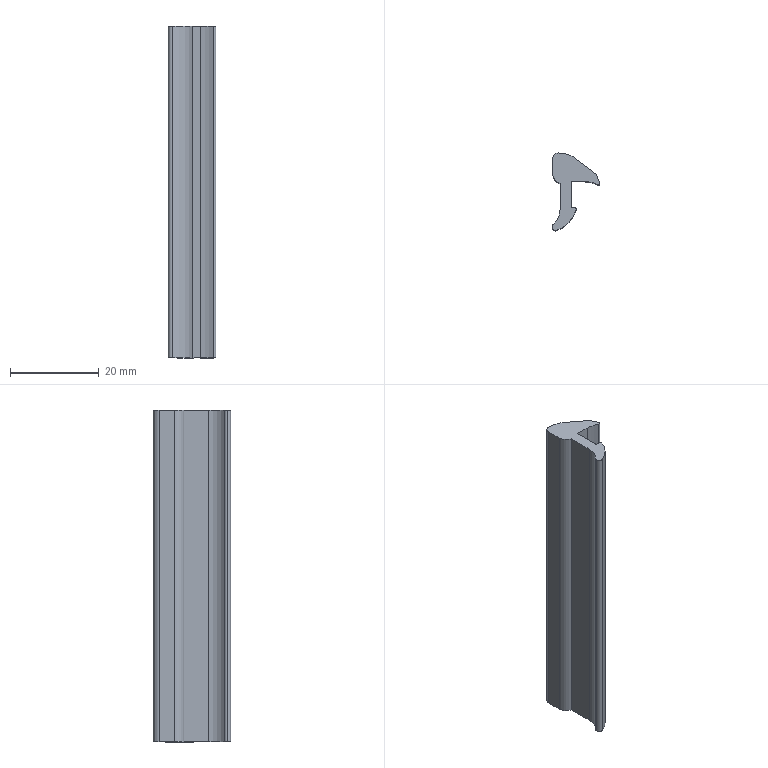Part | SolidWorks | features BaseBody 1, MoveFace 1 | 1 solid | 20 faces | box 10.8 x 17.5 x 75 mm | volume 5910 mm3 | cylinder 11 | plane 9 | commonest cylinder face diameters 1.6 x2 14 x2 0.4 x1 0.6 x1 0.8 x1 2.6 x1
STEP:
#1=CARTESIAN_POINT('',(-3.236,-11.055,-25.));
#2=VERTEX_POINT('',#1);
#3=CARTESIAN_POINT('',(-4.3,-10.3,-25.));
#4=VERTEX_POINT('',#3);
#5=CARTESIAN_POINT('',(-3.5,-10.3,-25.));
#6=DIRECTION('',(0.,0.,-1.));
#7=DIRECTION('',(1.,0.,0.));
#8=AXIS2_PLACEMENT_3D('',#5,#6,#7);
#9=CIRCLE('',#8,0.8);
#10=EDGE_CURVE('',#2,#4,#9,.T.);
#11=ORIENTED_EDGE('',*,*,#10,.T.);
#12=CARTESIAN_POINT('',(-4.3,-10.3,-100.));
#13=VERTEX_POINT('',#12);
#14=CARTESIAN_POINT('',(-4.3,-10.3,-100.));
#15=DIRECTION('',(0.,0.,-1.));
#16=VECTOR('',#15,1000.);
#17=LINE('',#14,#16);
#18=EDGE_CURVE('',#4,#13,#17,.T.);
#19=ORIENTED_EDGE('',*,*,#18,.T.);
#20=CARTESIAN_POINT('',(-3.236,-11.055,-100.));
#21=VERTEX_POINT('',#20);
#22=CARTESIAN_POINT('',(-3.5,-10.3,-100.));
#23=DIRECTION('',(0.,0.,1.));
#24=DIRECTION('',(-1.,0.,0.));
#25=AXIS2_PLACEMENT_3D('',#22,#23,#24);
#26=CIRCLE('',#25,0.8);
#27=EDGE_CURVE('',#13,#21,#26,.T.);
#28=ORIENTED_EDGE('',*,*,#27,.T.);
#29=CARTESIAN_POINT('',(-3.236,-11.055,-100.));
#30=DIRECTION('',(0.,0.,-1.));
#31=VECTOR('',#30,1000.);
#32=LINE('',#29,#31);
#33=EDGE_CURVE('',#2,#21,#32,.T.);
#34=ORIENTED_EDGE('',*,*,#33,.F.);
#35=EDGE_LOOP('',(#11,#19,#28,#34));
#36=FACE_OUTER_BOUND('',#35,.T.);
#37=CARTESIAN_POINT('',(-3.5,-10.3,-100.));
#38=DIRECTION('',(0.,0.,-1.));
#39=DIRECTION('',(-1.,0.,0.));
#40=AXIS2_PLACEMENT_3D('',#37,#38,#39);
#41=CYLINDRICAL_SURFACE('',#40,0.8);
#42=ADVANCED_FACE('',(#36),#41,.T.);
#43=CARTESIAN_POINT('',(1.184,-6.397,-100.));
#44=VERTEX_POINT('',#43);
#45=CARTESIAN_POINT('',(-5.702,-4.29,-100.));
#46=DIRECTION('',(0.,0.,1.));
#47=DIRECTION('',(-1.,0.,0.));
#48=AXIS2_PLACEMENT_3D('',#45,#46,#47);
#49=CIRCLE('',#48,7.201);
#50=EDGE_CURVE('',#21,#44,#49,.T.);
#51=ORIENTED_EDGE('',*,*,#50,.T.);
#52=CARTESIAN_POINT('',(1.184,-6.397,-25.));
#53=VERTEX_POINT('',#52);
#54=CARTESIAN_POINT('',(1.184,-6.397,-100.));
#55=DIRECTION('',(0.,0.,1.));
#56=VECTOR('',#55,1000.);
#57=LINE('',#54,#56);
#58=EDGE_CURVE('',#44,#53,#57,.T.);
#59=ORIENTED_EDGE('',*,*,#58,.T.);
#60=CARTESIAN_POINT('',(-5.702,-4.29,-25.));
#61=DIRECTION('',(0.,0.,-1.));
#62=DIRECTION('',(1.,0.,0.));
#63=AXIS2_PLACEMENT_3D('',#60,#61,#62);
#64=CIRCLE('',#63,7.201);
#65=EDGE_CURVE('',#53,#2,#64,.T.);
#66=ORIENTED_EDGE('',*,*,#65,.T.);
#67=ORIENTED_EDGE('',*,*,#33,.T.);
#68=EDGE_LOOP('',(#51,#59,#66,#67));
#69=FACE_OUTER_BOUND('',#68,.T.);
#70=CARTESIAN_POINT('',(-5.702,-4.29,-100.));
#71=DIRECTION('',(0.,0.,-1.));
#72=DIRECTION('',(-1.,0.,0.));
#73=AXIS2_PLACEMENT_3D('',#70,#71,#72);
#74=CYLINDRICAL_SURFACE('',#73,7.201);
#75=ADVANCED_FACE('',(#69),#74,.T.);
#76=CARTESIAN_POINT('',(0.9,-6.,-100.));
#77=VERTEX_POINT('',#76);
#78=CARTESIAN_POINT('',(0.9,-6.3,-100.));
#79=DIRECTION('',(0.,0.,1.));
#80=DIRECTION('',(-1.,0.,0.));
#81=AXIS2_PLACEMENT_3D('',#78,#79,#80);
#82=CIRCLE('',#81,0.3);
#83=EDGE_CURVE('',#44,#77,#82,.T.);
#84=ORIENTED_EDGE('',*,*,#83,.T.);
#85=CARTESIAN_POINT('',(0.9,-6.,-25.));
#86=VERTEX_POINT('',#85);
#87=CARTESIAN_POINT('',(0.9,-6.,-100.));
#88=DIRECTION('',(0.,0.,1.));
#89=VECTOR('',#88,1000.);
#90=LINE('',#87,#89);
#91=EDGE_CURVE('',#77,#86,#90,.T.);
#92=ORIENTED_EDGE('',*,*,#91,.T.);
#93=CARTESIAN_POINT('',(0.9,-6.3,-25.));
#94=DIRECTION('',(0.,0.,-1.));
#95=DIRECTION('',(1.,0.,0.));
#96=AXIS2_PLACEMENT_3D('',#93,#94,#95);
#97=CIRCLE('',#96,0.3);
#98=EDGE_CURVE('',#86,#53,#97,.T.);
#99=ORIENTED_EDGE('',*,*,#98,.T.);
#100=ORIENTED_EDGE('',*,*,#58,.F.);
#101=EDGE_LOOP('',(#84,#92,#99,#100));
#102=FACE_OUTER_BOUND('',#101,.T.);
#103=CARTESIAN_POINT('',(0.9,-6.3,-100.));
#104=DIRECTION('',(0.,0.,-1.));
#105=DIRECTION('',(-1.,0.,0.));
#106=AXIS2_PLACEMENT_3D('',#103,#104,#105);
#107=CYLINDRICAL_SURFACE('',#106,0.3);
#108=ADVANCED_FACE('',(#102),#107,.T.);
#109=CARTESIAN_POINT('',(-2.5,-0.5,-100.));
#110=VERTEX_POINT('',#109);
#111=CARTESIAN_POINT('',(-2.5,-6.153,-100.));
#112=VERTEX_POINT('',#111);
#113=CARTESIAN_POINT('',(-2.5,-6.397,-100.));
#114=DIRECTION('',(0.,-1.,0.));
#115=VECTOR('',#114,1000.);
#116=LINE('',#113,#115);
#117=EDGE_CURVE('',#110,#112,#116,.T.);
#118=ORIENTED_EDGE('',*,*,#117,.F.);
#119=CARTESIAN_POINT('',(-4.2,1.695,-100.));
#120=VERTEX_POINT('',#119);
#121=CARTESIAN_POINT('',(-1.701,1.875,-100.));
#122=DIRECTION('',(0.,0.,1.));
#123=DIRECTION('',(-1.,0.,0.));
#124=AXIS2_PLACEMENT_3D('',#121,#122,#123);
#125=CIRCLE('',#124,2.506);
#126=EDGE_CURVE('',#120,#110,#125,.T.);
#127=ORIENTED_EDGE('',*,*,#126,.F.);
#128=CARTESIAN_POINT('',(-4.2,5.1,-100.));
#129=VERTEX_POINT('',#128);
#130=CARTESIAN_POINT('',(-4.2,-6.397,-100.));
#131=DIRECTION('',(0.,-1.,0.));
#132=VECTOR('',#131,1000.);
#133=LINE('',#130,#132);
#134=EDGE_CURVE('',#129,#120,#133,.T.);
#135=ORIENTED_EDGE('',*,*,#134,.F.);
#136=CARTESIAN_POINT('',(-2.892,6.4,-100.));
#137=VERTEX_POINT('',#136);
#138=CARTESIAN_POINT('',(-2.9,5.1,-100.));
#139=DIRECTION('',(0.,0.,1.));
#140=DIRECTION('',(-1.,0.,0.));
#141=AXIS2_PLACEMENT_3D('',#138,#139,#140);
#142=CIRCLE('',#141,1.3);
#143=EDGE_CURVE('',#137,#129,#142,.T.);
#144=ORIENTED_EDGE('',*,*,#143,.F.);
#145=CARTESIAN_POINT('',(0.5,5.5,-100.));
#146=VERTEX_POINT('',#145);
#147=CARTESIAN_POINT('',(-2.934,-0.5999,-100.));
#148=DIRECTION('',(0.,0.,1.));
#149=DIRECTION('',(-1.,0.,0.));
#150=AXIS2_PLACEMENT_3D('',#147,#148,#149);
#151=CIRCLE('',#150,7.);
#152=EDGE_CURVE('',#146,#137,#151,.T.);
#153=ORIENTED_EDGE('',*,*,#152,.F.);
#154=CARTESIAN_POINT('',(5.5,1.7,-100.));
#155=VERTEX_POINT('',#154);
#156=CARTESIAN_POINT('',(5.5,1.7,-100.));
#157=DIRECTION('',(-0.7962,0.6051,0.));
#158=VECTOR('',#157,1000.);
#159=LINE('',#156,#158);
#160=EDGE_CURVE('',#155,#146,#159,.T.);
#161=ORIENTED_EDGE('',*,*,#160,.F.);
#162=CARTESIAN_POINT('',(6.458,-0.2215,-100.));
#163=VERTEX_POINT('',#162);
#164=CARTESIAN_POINT('',(6.458,-0.2215,-100.));
#165=DIRECTION('',(-0.4462,0.8949,0.));
#166=VECTOR('',#165,1000.);
#167=LINE('',#164,#166);
#168=EDGE_CURVE('',#163,#155,#167,.T.);
#169=ORIENTED_EDGE('',*,*,#168,.F.);
#170=CARTESIAN_POINT('',(5.895,-0.7433,-100.));
#171=VERTEX_POINT('',#170);
#172=CARTESIAN_POINT('',(6.1,-0.4,-100.));
#173=DIRECTION('',(0.,0.,1.));
#174=DIRECTION('',(-1.,0.,0.));
#175=AXIS2_PLACEMENT_3D('',#172,#173,#174);
#176=CIRCLE('',#175,0.4);
#177=EDGE_CURVE('',#171,#163,#176,.T.);
#178=ORIENTED_EDGE('',*,*,#177,.F.);
#179=CARTESIAN_POINT('',(3.,0.,-100.));
#180=VERTEX_POINT('',#179);
#181=CARTESIAN_POINT('',(2.746,-6.995,-100.));
#182=DIRECTION('',(0.,0.,-1.));
#183=DIRECTION('',(-1.,0.,0.));
#184=AXIS2_PLACEMENT_3D('',#181,#182,#183);
#185=CIRCLE('',#184,7.);
#186=EDGE_CURVE('',#180,#171,#185,.T.);
#187=ORIENTED_EDGE('',*,*,#186,.F.);
#188=CARTESIAN_POINT('',(0.,0.,-100.));
#189=VERTEX_POINT('',#188);
#190=CARTESIAN_POINT('',(-6.814,0.,-100.));
#191=DIRECTION('',(1.,0.,0.));
#192=VECTOR('',#191,1000.);
#193=LINE('',#190,#192);
#194=EDGE_CURVE('',#189,#180,#193,.T.);
#195=ORIENTED_EDGE('',*,*,#194,.F.);
#196=CARTESIAN_POINT('',(0.,-5.8,-100.));
#197=VERTEX_POINT('',#196);
#198=CARTESIAN_POINT('',(0.,-6.397,-100.));
#199=DIRECTION('',(0.,1.,0.));
#200=VECTOR('',#199,1000.);
#201=LINE('',#198,#200);
#202=EDGE_CURVE('',#197,#189,#201,.T.);
#203=ORIENTED_EDGE('',*,*,#202,.F.);
#204=CARTESIAN_POINT('',(0.2,-6.,-100.));
#205=VERTEX_POINT('',#204);
#206=CARTESIAN_POINT('',(0.2,-5.8,-100.));
#207=DIRECTION('',(0.,0.,1.));
#208=DIRECTION('',(-1.,0.,0.));
#209=AXIS2_PLACEMENT_3D('',#206,#207,#208);
#210=CIRCLE('',#209,0.2);
#211=EDGE_CURVE('',#197,#205,#210,.T.);
#212=ORIENTED_EDGE('',*,*,#211,.T.);
#213=CARTESIAN_POINT('',(-6.814,-6.,-100.));
#214=DIRECTION('',(-1.,0.,0.));
#215=VECTOR('',#214,1000.);
#216=LINE('',#213,#215);
#217=EDGE_CURVE('',#77,#205,#216,.T.);
#218=ORIENTED_EDGE('',*,*,#217,.F.);
#219=ORIENTED_EDGE('',*,*,#83,.F.);
#220=ORIENTED_EDGE('',*,*,#50,.F.);
#221=ORIENTED_EDGE('',*,*,#27,.F.);
#222=CARTESIAN_POINT('',(-3.998,-9.674,-100.));
#223=VERTEX_POINT('',#222);
#224=CARTESIAN_POINT('',(-3.5,-10.3,-100.));
#225=DIRECTION('',(0.,0.,1.));
#226=DIRECTION('',(-1.,0.,0.));
#227=AXIS2_PLACEMENT_3D('',#224,#225,#226);
#228=CIRCLE('',#227,0.8);
#229=EDGE_CURVE('',#223,#13,#228,.T.);
#230=ORIENTED_EDGE('',*,*,#229,.F.);
#231=CARTESIAN_POINT('',(-6.814,-6.397,-100.));
#232=DIRECTION('',(0.,0.,-1.));
#233=DIRECTION('',(-1.,0.,0.));
#234=AXIS2_PLACEMENT_3D('',#231,#232,#233);
#235=CIRCLE('',#234,4.321);
#236=EDGE_CURVE('',#112,#223,#235,.T.);
#237=ORIENTED_EDGE('',*,*,#236,.F.);
#238=EDGE_LOOP('',(#118,#127,#135,#144,#153,#161,#169,#178,#187,#195,#203,#212,#218,#219,#220,#221,#230,#237));
#239=FACE_OUTER_BOUND('',#238,.T.);
#240=CARTESIAN_POINT('',(-6.814,-6.397,-100.));
#241=DIRECTION('',(0.,0.,1.));
#242=DIRECTION('',(1.,0.,0.));
#243=AXIS2_PLACEMENT_3D('',#240,#241,#242);
#244=PLANE('',#243);
#245=ADVANCED_FACE('',(#239),#244,.F.);
#246=ORIENTED_EDGE('',*,*,#18,.F.);
#247=CARTESIAN_POINT('',(-3.998,-9.674,-25.));
#248=VERTEX_POINT('',#247);
#249=CARTESIAN_POINT('',(-3.5,-10.3,-25.));
#250=DIRECTION('',(0.,0.,-1.));
#251=DIRECTION('',(1.,0.,0.));
#252=AXIS2_PLACEMENT_3D('',#249,#250,#251);
#253=CIRCLE('',#252,0.8);
#254=EDGE_CURVE('',#4,#248,#253,.T.);
#255=ORIENTED_EDGE('',*,*,#254,.T.);
#256=CARTESIAN_POINT('',(-3.998,-9.674,-100.));
#257=DIRECTION('',(0.,0.,-1.));
#258=VECTOR('',#257,1000.);
#259=LINE('',#256,#258);
#260=EDGE_CURVE('',#248,#223,#259,.T.);
#261=ORIENTED_EDGE('',*,*,#260,.T.);
#262=ORIENTED_EDGE('',*,*,#229,.T.);
#263=EDGE_LOOP('',(#246,#255,#261,#262));
#264=FACE_OUTER_BOUND('',#263,.T.);
#265=CARTESIAN_POINT('',(-3.5,-10.3,-100.));
#266=DIRECTION('',(0.,0.,-1.));
#267=DIRECTION('',(-1.,0.,0.));
#268=AXIS2_PLACEMENT_3D('',#265,#266,#267);
#269=CYLINDRICAL_SURFACE('',#268,0.8);
#270=ADVANCED_FACE('',(#264),#269,.T.);
#271=CARTESIAN_POINT('',(-4.2,1.695,-25.));
#272=VERTEX_POINT('',#271);
#273=CARTESIAN_POINT('',(-2.5,-0.5,-25.));
#274=VERTEX_POINT('',#273);
#275=CARTESIAN_POINT('',(-1.701,1.875,-25.));
#276=DIRECTION('',(0.,0.,1.));
#277=DIRECTION('',(1.,0.,0.));
#278=AXIS2_PLACEMENT_3D('',#275,#276,#277);
#279=CIRCLE('',#278,2.506);
#280=EDGE_CURVE('',#272,#274,#279,.T.);
#281=ORIENTED_EDGE('',*,*,#280,.T.);
#282=CARTESIAN_POINT('',(-2.5,-6.153,-25.));
#283=VERTEX_POINT('',#282);
#284=CARTESIAN_POINT('',(-2.5,-6.397,-25.));
#285=DIRECTION('',(0.,-1.,0.));
#286=VECTOR('',#285,1000.);
#287=LINE('',#284,#286);
#288=EDGE_CURVE('',#274,#283,#287,.T.);
#289=ORIENTED_EDGE('',*,*,#288,.T.);
#290=CARTESIAN_POINT('',(-6.814,-6.397,-25.));
#291=DIRECTION('',(0.,0.,-1.));
#292=DIRECTION('',(1.,0.,0.));
#293=AXIS2_PLACEMENT_3D('',#290,#291,#292);
#294=CIRCLE('',#293,4.321);
#295=EDGE_CURVE('',#283,#248,#294,.T.);
#296=ORIENTED_EDGE('',*,*,#295,.T.);
#297=ORIENTED_EDGE('',*,*,#254,.F.);
#298=ORIENTED_EDGE('',*,*,#10,.F.);
#299=ORIENTED_EDGE('',*,*,#65,.F.);
#300=ORIENTED_EDGE('',*,*,#98,.F.);
#301=CARTESIAN_POINT('',(0.2,-6.,-25.));
#302=VERTEX_POINT('',#301);
#303=CARTESIAN_POINT('',(-6.814,-6.,-25.));
#304=DIRECTION('',(-1.,0.,0.));
#305=VECTOR('',#304,1000.);
#306=LINE('',#303,#305);
#307=EDGE_CURVE('',#86,#302,#306,.T.);
#308=ORIENTED_EDGE('',*,*,#307,.T.);
#309=CARTESIAN_POINT('',(0.,-5.8,-25.));
#310=VERTEX_POINT('',#309);
#311=CARTESIAN_POINT('',(0.2,-5.8,-25.));
#312=DIRECTION('',(0.,0.,-1.));
#313=DIRECTION('',(1.,0.,0.));
#314=AXIS2_PLACEMENT_3D('',#311,#312,#313);
#315=CIRCLE('',#314,0.2);
#316=EDGE_CURVE('',#302,#310,#315,.T.);
#317=ORIENTED_EDGE('',*,*,#316,.T.);
#318=CARTESIAN_POINT('',(0.,0.,-25.));
#319=VERTEX_POINT('',#318);
#320=CARTESIAN_POINT('',(0.,-6.397,-25.));
#321=DIRECTION('',(0.,1.,0.));
#322=VECTOR('',#321,1000.);
#323=LINE('',#320,#322);
#324=EDGE_CURVE('',#310,#319,#323,.T.);
#325=ORIENTED_EDGE('',*,*,#324,.T.);
#326=CARTESIAN_POINT('',(3.,0.,-25.));
#327=VERTEX_POINT('',#326);
#328=CARTESIAN_POINT('',(-6.814,0.,-25.));
#329=DIRECTION('',(1.,0.,0.));
#330=VECTOR('',#329,1000.);
#331=LINE('',#328,#330);
#332=EDGE_CURVE('',#319,#327,#331,.T.);
#333=ORIENTED_EDGE('',*,*,#332,.T.);
#334=CARTESIAN_POINT('',(5.895,-0.7433,-25.));
#335=VERTEX_POINT('',#334);
#336=CARTESIAN_POINT('',(2.746,-6.995,-25.));
#337=DIRECTION('',(0.,0.,-1.));
#338=DIRECTION('',(1.,0.,0.));
#339=AXIS2_PLACEMENT_3D('',#336,#337,#338);
#340=CIRCLE('',#339,7.);
#341=EDGE_CURVE('',#327,#335,#340,.T.);
#342=ORIENTED_EDGE('',*,*,#341,.T.);
#343=CARTESIAN_POINT('',(6.458,-0.2215,-25.));
#344=VERTEX_POINT('',#343);
#345=CARTESIAN_POINT('',(6.1,-0.4,-25.));
#346=DIRECTION('',(0.,0.,-1.));
#347=DIRECTION('',(1.,0.,0.));
#348=AXIS2_PLACEMENT_3D('',#345,#346,#347);
#349=CIRCLE('',#348,0.4);
#350=EDGE_CURVE('',#344,#335,#349,.T.);
#351=ORIENTED_EDGE('',*,*,#350,.F.);
#352=CARTESIAN_POINT('',(5.5,1.7,-25.));
#353=VERTEX_POINT('',#352);
#354=CARTESIAN_POINT('',(6.282,0.1323,-25.));
#355=DIRECTION('',(-0.4462,0.8949,0.));
#356=VECTOR('',#355,1000.);
#357=LINE('',#354,#356);
#358=EDGE_CURVE('',#344,#353,#357,.T.);
#359=ORIENTED_EDGE('',*,*,#358,.T.);
#360=CARTESIAN_POINT('',(0.5,5.5,-25.));
#361=VERTEX_POINT('',#360);
#362=CARTESIAN_POINT('',(1.595,4.668,-25.));
#363=DIRECTION('',(-0.7962,0.6051,0.));
#364=VECTOR('',#363,1000.);
#365=LINE('',#362,#364);
#366=EDGE_CURVE('',#353,#361,#365,.T.);
#367=ORIENTED_EDGE('',*,*,#366,.T.);
#368=CARTESIAN_POINT('',(-2.892,6.4,-25.));
#369=VERTEX_POINT('',#368);
#370=CARTESIAN_POINT('',(-2.934,-0.5999,-25.));
#371=DIRECTION('',(0.,0.,1.));
#372=DIRECTION('',(1.,0.,0.));
#373=AXIS2_PLACEMENT_3D('',#370,#371,#372);
#374=CIRCLE('',#373,7.);
#375=EDGE_CURVE('',#361,#369,#374,.T.);
#376=ORIENTED_EDGE('',*,*,#375,.T.);
#377=CARTESIAN_POINT('',(-4.2,5.1,-25.));
#378=VERTEX_POINT('',#377);
#379=CARTESIAN_POINT('',(-2.9,5.1,-25.));
#380=DIRECTION('',(0.,0.,1.));
#381=DIRECTION('',(1.,0.,0.));
#382=AXIS2_PLACEMENT_3D('',#379,#380,#381);
#383=CIRCLE('',#382,1.3);
#384=EDGE_CURVE('',#369,#378,#383,.T.);
#385=ORIENTED_EDGE('',*,*,#384,.T.);
#386=CARTESIAN_POINT('',(-4.2,-6.397,-25.));
#387=DIRECTION('',(0.,-1.,0.));
#388=VECTOR('',#387,1000.);
#389=LINE('',#386,#388);
#390=EDGE_CURVE('',#378,#272,#389,.T.);
#391=ORIENTED_EDGE('',*,*,#390,.T.);
#392=EDGE_LOOP('',(#281,#289,#296,#297,#298,#299,#300,#308,#317,#325,#333,#342,#351,#359,#367,#376,#385,#391));
#393=FACE_OUTER_BOUND('',#392,.T.);
#394=CARTESIAN_POINT('',(-6.814,-6.397,-25.));
#395=DIRECTION('',(0.,0.,1.));
#396=DIRECTION('',(1.,0.,0.));
#397=AXIS2_PLACEMENT_3D('',#394,#395,#396);
#398=PLANE('',#397);
#399=ADVANCED_FACE('',(#393),#398,.T.);
#400=ORIENTED_EDGE('',*,*,#217,.T.);
#401=CARTESIAN_POINT('',(0.2,-6.,-100.));
#402=DIRECTION('',(0.,0.,1.));
#403=VECTOR('',#402,1000.);
#404=LINE('',#401,#403);
#405=EDGE_CURVE('',#205,#302,#404,.T.);
#406=ORIENTED_EDGE('',*,*,#405,.T.);
#407=ORIENTED_EDGE('',*,*,#307,.F.);
#408=ORIENTED_EDGE('',*,*,#91,.F.);
#409=EDGE_LOOP('',(#400,#406,#407,#408));
#410=FACE_OUTER_BOUND('',#409,.T.);
#411=CARTESIAN_POINT('',(0.9,-6.,-100.));
#412=DIRECTION('',(0.,1.,0.));
#413=DIRECTION('',(0.,0.,1.));
#414=AXIS2_PLACEMENT_3D('',#411,#412,#413);
#415=PLANE('',#414);
#416=ADVANCED_FACE('',(#410),#415,.T.);
#417=CARTESIAN_POINT('',(-2.5,-6.153,-100.));
#418=DIRECTION('',(0.,0.,1.));
#419=VECTOR('',#418,1000.);
#420=LINE('',#417,#419);
#421=EDGE_CURVE('',#112,#283,#420,.T.);
#422=ORIENTED_EDGE('',*,*,#421,.F.);
#423=ORIENTED_EDGE('',*,*,#236,.T.);
#424=ORIENTED_EDGE('',*,*,#260,.F.);
#425=ORIENTED_EDGE('',*,*,#295,.F.);
#426=EDGE_LOOP('',(#422,#423,#424,#425));
#427=FACE_OUTER_BOUND('',#426,.T.);
#428=CARTESIAN_POINT('',(-6.814,-6.397,-100.));
#429=DIRECTION('',(0.,0.,-1.));
#430=DIRECTION('',(-1.,0.,0.));
#431=AXIS2_PLACEMENT_3D('',#428,#429,#430);
#432=CYLINDRICAL_SURFACE('',#431,4.321);
#433=ADVANCED_FACE('',(#427),#432,.F.);
#434=ORIENTED_EDGE('',*,*,#117,.T.);
#435=ORIENTED_EDGE('',*,*,#421,.T.);
#436=ORIENTED_EDGE('',*,*,#288,.F.);
#437=CARTESIAN_POINT('',(-2.5,-0.5,-100.));
#438=DIRECTION('',(0.,0.,-1.));
#439=VECTOR('',#438,1000.);
#440=LINE('',#437,#439);
#441=EDGE_CURVE('',#274,#110,#440,.T.);
#442=ORIENTED_EDGE('',*,*,#441,.T.);
#443=EDGE_LOOP('',(#434,#435,#436,#442));
#444=FACE_OUTER_BOUND('',#443,.T.);
#445=CARTESIAN_POINT('',(-2.5,-0.5,-100.));
#446=DIRECTION('',(-1.,0.,0.));
#447=DIRECTION('',(0.,0.,1.));
#448=AXIS2_PLACEMENT_3D('',#445,#446,#447);
#449=PLANE('',#448);
#450=ADVANCED_FACE('',(#444),#449,.T.);
#451=ORIENTED_EDGE('',*,*,#126,.T.);
#452=ORIENTED_EDGE('',*,*,#441,.F.);
#453=ORIENTED_EDGE('',*,*,#280,.F.);
#454=CARTESIAN_POINT('',(-4.2,1.695,-100.));
#455=DIRECTION('',(0.,0.,-1.));
#456=VECTOR('',#455,1000.);
#457=LINE('',#454,#456);
#458=EDGE_CURVE('',#272,#120,#457,.T.);
#459=ORIENTED_EDGE('',*,*,#458,.T.);
#460=EDGE_LOOP('',(#451,#452,#453,#459));
#461=FACE_OUTER_BOUND('',#460,.T.);
#462=CARTESIAN_POINT('',(-1.701,1.875,-100.));
#463=DIRECTION('',(0.,0.,-1.));
#464=DIRECTION('',(-1.,0.,0.));
#465=AXIS2_PLACEMENT_3D('',#462,#463,#464);
#466=CYLINDRICAL_SURFACE('',#465,2.506);
#467=ADVANCED_FACE('',(#461),#466,.T.);
#468=ORIENTED_EDGE('',*,*,#134,.T.);
#469=ORIENTED_EDGE('',*,*,#458,.F.);
#470=ORIENTED_EDGE('',*,*,#390,.F.);
#471=CARTESIAN_POINT('',(-4.2,5.1,-100.));
#472=DIRECTION('',(0.,0.,-1.));
#473=VECTOR('',#472,1000.);
#474=LINE('',#471,#473);
#475=EDGE_CURVE('',#378,#129,#474,.T.);
#476=ORIENTED_EDGE('',*,*,#475,.T.);
#477=EDGE_LOOP('',(#468,#469,#470,#476));
#478=FACE_OUTER_BOUND('',#477,.T.);
#479=CARTESIAN_POINT('',(-4.2,5.1,-100.));
#480=DIRECTION('',(-1.,0.,0.));
#481=DIRECTION('',(0.,0.,1.));
#482=AXIS2_PLACEMENT_3D('',#479,#480,#481);
#483=PLANE('',#482);
#484=ADVANCED_FACE('',(#478),#483,.T.);
#485=ORIENTED_EDGE('',*,*,#143,.T.);
#486=ORIENTED_EDGE('',*,*,#475,.F.);
#487=ORIENTED_EDGE('',*,*,#384,.F.);
#488=CARTESIAN_POINT('',(-2.892,6.4,-100.));
#489=DIRECTION('',(0.,0.,-1.));
#490=VECTOR('',#489,1000.);
#491=LINE('',#488,#490);
#492=EDGE_CURVE('',#369,#137,#491,.T.);
#493=ORIENTED_EDGE('',*,*,#492,.T.);
#494=EDGE_LOOP('',(#485,#486,#487,#493));
#495=FACE_OUTER_BOUND('',#494,.T.);
#496=CARTESIAN_POINT('',(-2.9,5.1,-100.));
#497=DIRECTION('',(0.,0.,-1.));
#498=DIRECTION('',(-1.,0.,0.));
#499=AXIS2_PLACEMENT_3D('',#496,#497,#498);
#500=CYLINDRICAL_SURFACE('',#499,1.3);
#501=ADVANCED_FACE('',(#495),#500,.T.);
#502=ORIENTED_EDGE('',*,*,#152,.T.);
#503=ORIENTED_EDGE('',*,*,#492,.F.);
#504=ORIENTED_EDGE('',*,*,#375,.F.);
#505=CARTESIAN_POINT('',(0.5,5.5,-100.));
#506=DIRECTION('',(0.,0.,-1.));
#507=VECTOR('',#506,1000.);
#508=LINE('',#505,#507);
#509=EDGE_CURVE('',#361,#146,#508,.T.);
#510=ORIENTED_EDGE('',*,*,#509,.T.);
#511=EDGE_LOOP('',(#502,#503,#504,#510));
#512=FACE_OUTER_BOUND('',#511,.T.);
#513=CARTESIAN_POINT('',(-2.934,-0.5999,-100.));
#514=DIRECTION('',(0.,0.,-1.));
#515=DIRECTION('',(-1.,0.,0.));
#516=AXIS2_PLACEMENT_3D('',#513,#514,#515);
#517=CYLINDRICAL_SURFACE('',#516,7.);
#518=ADVANCED_FACE('',(#512),#517,.T.);
#519=ORIENTED_EDGE('',*,*,#160,.T.);
#520=ORIENTED_EDGE('',*,*,#509,.F.);
#521=ORIENTED_EDGE('',*,*,#366,.F.);
#522=CARTESIAN_POINT('',(5.5,1.7,-100.));
#523=DIRECTION('',(0.,0.,-1.));
#524=VECTOR('',#523,1000.);
#525=LINE('',#522,#524);
#526=EDGE_CURVE('',#353,#155,#525,.T.);
#527=ORIENTED_EDGE('',*,*,#526,.T.);
#528=EDGE_LOOP('',(#519,#520,#521,#527));
#529=FACE_OUTER_BOUND('',#528,.T.);
#530=CARTESIAN_POINT('',(5.5,1.7,-100.));
#531=DIRECTION('',(0.6051,0.7962,0.));
#532=DIRECTION('',(-0.7962,0.6051,0.));
#533=AXIS2_PLACEMENT_3D('',#530,#531,#532);
#534=PLANE('',#533);
#535=ADVANCED_FACE('',(#529),#534,.T.);
#536=ORIENTED_EDGE('',*,*,#168,.T.);
#537=ORIENTED_EDGE('',*,*,#526,.F.);
#538=ORIENTED_EDGE('',*,*,#358,.F.);
#539=CARTESIAN_POINT('',(6.458,-0.2215,-100.));
#540=DIRECTION('',(0.,0.,-1.));
#541=VECTOR('',#540,1000.);
#542=LINE('',#539,#541);
#543=EDGE_CURVE('',#344,#163,#542,.T.);
#544=ORIENTED_EDGE('',*,*,#543,.T.);
#545=EDGE_LOOP('',(#536,#537,#538,#544));
#546=FACE_OUTER_BOUND('',#545,.T.);
#547=CARTESIAN_POINT('',(6.458,-0.2215,-100.));
#548=DIRECTION('',(0.8949,0.4462,0.));
#549=DIRECTION('',(-0.4462,0.8949,0.));
#550=AXIS2_PLACEMENT_3D('',#547,#548,#549);
#551=PLANE('',#550);
#552=ADVANCED_FACE('',(#546),#551,.T.);
#553=CARTESIAN_POINT('',(3.,0.,-100.));
#554=DIRECTION('',(0.,0.,1.));
#555=VECTOR('',#554,1000.);
#556=LINE('',#553,#555);
#557=EDGE_CURVE('',#180,#327,#556,.T.);
#558=ORIENTED_EDGE('',*,*,#557,.F.);
#559=ORIENTED_EDGE('',*,*,#186,.T.);
#560=CARTESIAN_POINT('',(5.895,-0.7433,-100.));
#561=DIRECTION('',(0.,0.,-1.));
#562=VECTOR('',#561,1000.);
#563=LINE('',#560,#562);
#564=EDGE_CURVE('',#335,#171,#563,.T.);
#565=ORIENTED_EDGE('',*,*,#564,.F.);
#566=ORIENTED_EDGE('',*,*,#341,.F.);
#567=EDGE_LOOP('',(#558,#559,#565,#566));
#568=FACE_OUTER_BOUND('',#567,.T.);
#569=CARTESIAN_POINT('',(2.746,-6.995,-100.));
#570=DIRECTION('',(0.,0.,-1.));
#571=DIRECTION('',(-1.,0.,0.));
#572=AXIS2_PLACEMENT_3D('',#569,#570,#571);
#573=CYLINDRICAL_SURFACE('',#572,7.);
#574=ADVANCED_FACE('',(#568),#573,.F.);
#575=ORIENTED_EDGE('',*,*,#194,.T.);
#576=ORIENTED_EDGE('',*,*,#557,.T.);
#577=ORIENTED_EDGE('',*,*,#332,.F.);
#578=CARTESIAN_POINT('',(0.,0.,-100.));
#579=DIRECTION('',(0.,0.,-1.));
#580=VECTOR('',#579,1000.);
#581=LINE('',#578,#580);
#582=EDGE_CURVE('',#319,#189,#581,.T.);
#583=ORIENTED_EDGE('',*,*,#582,.T.);
#584=EDGE_LOOP('',(#575,#576,#577,#583));
#585=FACE_OUTER_BOUND('',#584,.T.);
#586=CARTESIAN_POINT('',(0.,0.,-100.));
#587=DIRECTION('',(0.,-1.,0.));
#588=DIRECTION('',(0.,0.,-1.));
#589=AXIS2_PLACEMENT_3D('',#586,#587,#588);
#590=PLANE('',#589);
#591=ADVANCED_FACE('',(#585),#590,.T.);
#592=ORIENTED_EDGE('',*,*,#202,.T.);
#593=ORIENTED_EDGE('',*,*,#582,.F.);
#594=ORIENTED_EDGE('',*,*,#324,.F.);
#595=CARTESIAN_POINT('',(0.,-5.8,-100.));
#596=DIRECTION('',(0.,0.,-1.));
#597=VECTOR('',#596,1000.);
#598=LINE('',#595,#597);
#599=EDGE_CURVE('',#310,#197,#598,.T.);
#600=ORIENTED_EDGE('',*,*,#599,.T.);
#601=EDGE_LOOP('',(#592,#593,#594,#600));
#602=FACE_OUTER_BOUND('',#601,.T.);
#603=CARTESIAN_POINT('',(0.,-5.8,-100.));
#604=DIRECTION('',(1.,0.,0.));
#605=DIRECTION('',(0.,0.,-1.));
#606=AXIS2_PLACEMENT_3D('',#603,#604,#605);
#607=PLANE('',#606);
#608=ADVANCED_FACE('',(#602),#607,.T.);
#609=ORIENTED_EDGE('',*,*,#405,.F.);
#610=ORIENTED_EDGE('',*,*,#211,.F.);
#611=ORIENTED_EDGE('',*,*,#599,.F.);
#612=ORIENTED_EDGE('',*,*,#316,.F.);
#613=EDGE_LOOP('',(#609,#610,#611,#612));
#614=FACE_OUTER_BOUND('',#613,.T.);
#615=CARTESIAN_POINT('',(0.2,-5.8,-100.));
#616=DIRECTION('',(0.,0.,-1.));
#617=DIRECTION('',(-1.,0.,0.));
#618=AXIS2_PLACEMENT_3D('',#615,#616,#617);
#619=CYLINDRICAL_SURFACE('',#618,0.2);
#620=ADVANCED_FACE('',(#614),#619,.F.);
#621=ORIENTED_EDGE('',*,*,#177,.T.);
#622=ORIENTED_EDGE('',*,*,#543,.F.);
#623=ORIENTED_EDGE('',*,*,#350,.T.);
#624=ORIENTED_EDGE('',*,*,#564,.T.);
#625=EDGE_LOOP('',(#621,#622,#623,#624));
#626=FACE_OUTER_BOUND('',#625,.T.);
#627=CARTESIAN_POINT('',(6.1,-0.4,-100.));
#628=DIRECTION('',(0.,0.,-1.));
#629=DIRECTION('',(-1.,0.,0.));
#630=AXIS2_PLACEMENT_3D('',#627,#628,#629);
#631=CYLINDRICAL_SURFACE('',#630,0.4);
#632=ADVANCED_FACE('',(#626),#631,.T.);
#633=CLOSED_SHELL('',(#42,#75,#108,#245,#270,#399,#416,#433,#450,#467,#484,#501,#518,#535,#552,#574,#591,#608,#620,#632));
#634=MANIFOLD_SOLID_BREP('',#633);
#635=CARTESIAN_POINT('',(0.,0.,0.));
#636=DIRECTION('',(0.,0.,1.));
#637=DIRECTION('',(1.,0.,0.));
#638=AXIS2_PLACEMENT_3D('',#635,#636,#637);
#639=(LENGTH_UNIT()NAMED_UNIT(*)SI_UNIT(.MILLI.,.METRE.));
#640=UNCERTAINTY_MEASURE_WITH_UNIT(LENGTH_MEASURE(0.00001),#639,'','');
#641=(NAMED_UNIT(*)PLANE_ANGLE_UNIT()SI_UNIT($,.RADIAN.));
#642=(NAMED_UNIT(*)SI_UNIT($,.STERADIAN.)SOLID_ANGLE_UNIT());
#643=(GEOMETRIC_REPRESENTATION_CONTEXT(3)GLOBAL_UNCERTAINTY_ASSIGNED_CONTEXT((#640))GLOBAL_UNIT_ASSIGNED_CONTEXT((#639,#641,#642))REPRESENTATION_CONTEXT('',''));
#644=ADVANCED_BREP_SHAPE_REPRESENTATION('',(#634,#638),#643);